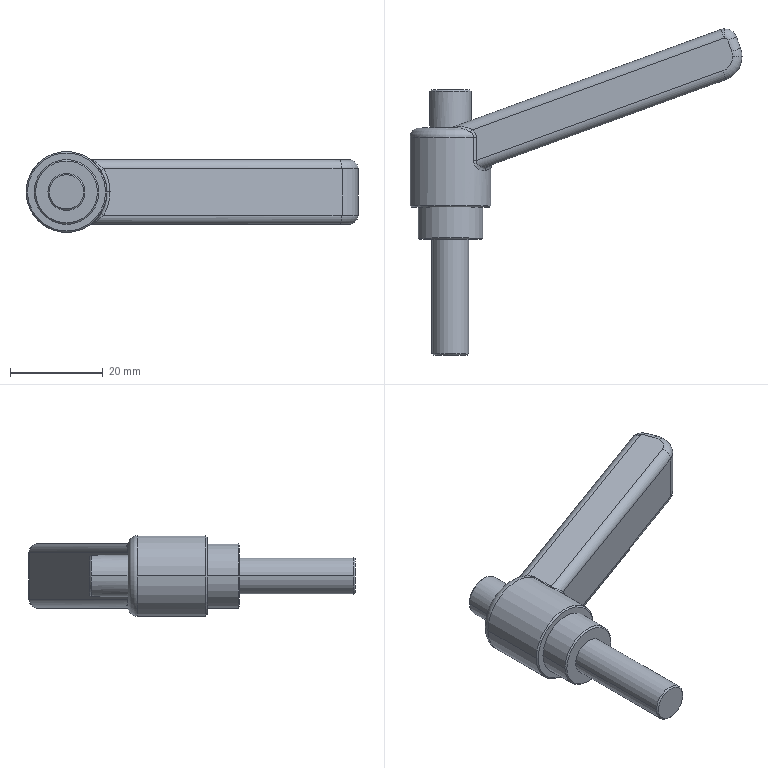Part | NX | 1 solid | 65 faces | box 71.75 x 70.5 x 17.5 mm | volume 15278 mm3 | cylinder 21 | plane 17 | spline 10 | torus 9 | cone 8 | commonest cylinder face diameters 4 x6 2 x4 8 x2 9 x2 10.5 x2 14 x2